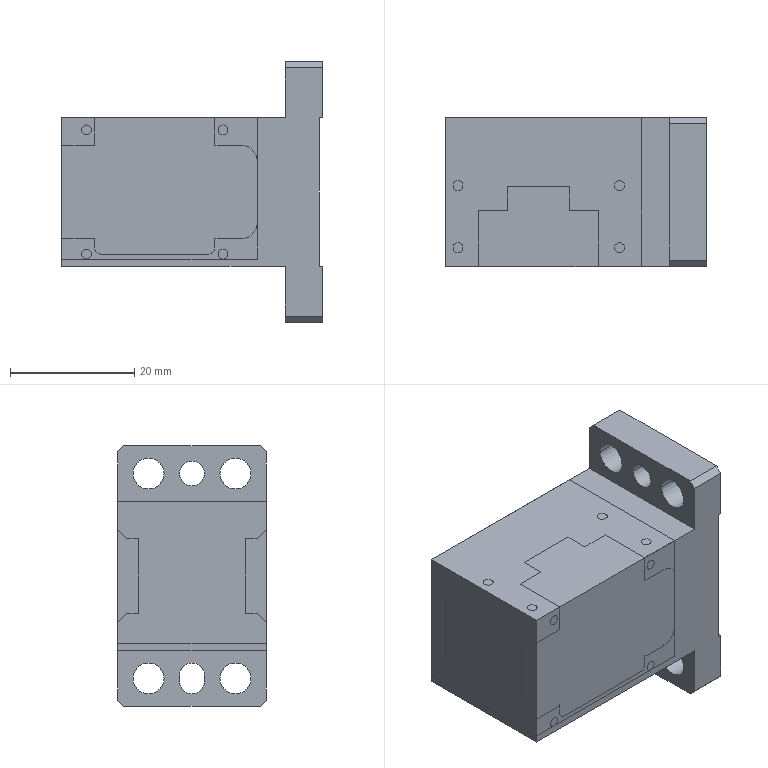NC program | NX | posted with a generic post | part box 42 x 24 x 42 mm
Whole program, first 1893 of 2020 lines:
N10 G17 G21 G94 G90
(DRILLING_COPY_2 , TOOL : ZXZ)
N12 T08 M6
N14 G54
N16 G17 G0 G90 X10. Y-17. B0. C0. S5000 M3
N18 G43 Z30. H8
N20 G94 G81 G98 Z-1.1 F250. R3.
N22 X-10.
N24 Y5.
N26 X10.
N28 G80
N30 G0 X10. Y5. Z30.
N32 M5
(DRILLING_COPY_COPY_1 , TOOL : 1.6ZT)
N34 T16 M6
N36 G54
N38 G17 G0 G90 X10. Y-17. B0. C0. S2000 M3
N40 G43 Z30. H16
N42 G94 G83 G98 Z-5.681 F100. Q2. R3.
N44 X-10.
N46 Y5.
N48 X10.
N50 G80
N52 G0 X10. Y5. Z30.
N54 M5
(FLOOR_WALL_1_COPY_COPY , TOOL : D6)
N56 T06 M6
N58 G54
N60 G17 G0 G90 X1.212 Y-25.5 B0. C0. S4500 M3
N62 G43 Z30. H6
N64 Z1.45
N66 G94 G1 Z-0.05 F1000.
N68 X0.52 Y-24.3
N70 G3 X0. Y-24. R0.6
N72 G1 X-3. F2000.
N74 Y-15.
N76 X3.
N78 Y-24.
N80 X0.
N82 Y-21.
N84 Y-18.
N86 Y-21.
N88 G3 X0.3 Y-21.52 R0.6
N90 G1 Y-25.5
N92 Z1.45
N94 G0 X1.212 Z1.35
N96 G1 Z-0.15 F1000.
N98 X0.52 Y-24.3
N100 G3 X0. Y-24. R0.6
N102 G1 X-3. F2000.
N104 Y-15.
N106 X3.
N108 Y-24.
N110 X0.
N112 Y-21.
N114 Y-18.
N116 Y-21.
N118 G3 X0.3 Y-21.52 R0.6
N120 G1 Y-25.5
N122 Z1.35
N124 G0 X1.212 Z1.25
N126 G1 Z-0.25 F1000.
N128 X0.52 Y-24.3
N130 G3 X0. Y-24. R0.6
N132 G1 X-3. F2000.
N134 Y-15.
N136 X3.
N138 Y-24.
N140 X0.
N142 Y-21.
N144 Y-18.
N146 Y-21.
N148 G3 X0.3 Y-21.52 R0.6
N150 G1 Y-25.5
N152 Z1.25
N154 G0 X1.212 Z1.15
N156 G1 Z-0.35 F1000.
N158 X0.52 Y-24.3
N160 G3 X0. Y-24. R0.6
N162 G1 X-3. F2000.
N164 Y-15.
N166 X3.
N168 Y-24.
N170 X0.
N172 Y-21.
N174 Y-18.
N176 Y-21.
N178 G3 X0.3 Y-21.52 R0.6
N180 G1 Y-25.5
N182 Z1.15
N184 G0 X1.212 Z1.05
N186 G1 Z-0.45 F1000.
N188 X0.52 Y-24.3
N190 G3 X0. Y-24. R0.6
N192 G1 X-3. F2000.
N194 Y-15.
N196 X3.
N198 Y-24.
N200 X0.
N202 Y-21.
N204 Y-18.
N206 Y-21.
N208 G3 X0.3 Y-21.52 R0.6
N210 G1 Y-25.5
N212 Z1.05
N214 G0 X1.212 Z0.95
N216 G1 Z-0.55 F1000.
N218 X0.52 Y-24.3
N220 G3 X0. Y-24. R0.6
N222 G1 X-3. F2000.
N224 Y-15.
N226 X3.
N228 Y-24.
N230 X0.
N232 Y-21.
N234 Y-18.
N236 Y-21.
N238 G3 X0.3 Y-21.52 R0.6
N240 G1 Y-25.5
N242 Z0.95
N244 G0 X1.212 Z0.85
N246 G1 Z-0.65 F1000.
N248 X0.52 Y-24.3
N250 G3 X0. Y-24. R0.6
N252 G1 X-3. F2000.
N254 Y-15.
N256 X3.
N258 Y-24.
N260 X0.
N262 Y-21.
N264 Y-18.
N266 Y-21.
N268 G3 X0.3 Y-21.52 R0.6
N270 G1 Y-25.5
N272 Z0.85
N274 G0 X1.212 Z0.75
N276 G1 Z-0.75 F1000.
N278 X0.52 Y-24.3
N280 G3 X0. Y-24. R0.6
N282 G1 X-3. F2000.
N284 Y-15.
N286 X3.
N288 Y-24.
N290 X0.
N292 Y-21.
N294 Y-18.
N296 Y-21.
N298 G3 X0.3 Y-21.52 R0.6
N300 G1 Y-25.5
N302 Z0.75
N304 G0 X1.212 Z0.65
N306 G1 Z-0.85 F1000.
N308 X0.52 Y-24.3
N310 G3 X0. Y-24. R0.6
N312 G1 X-3. F2000.
N314 Y-15.
N316 X3.
N318 Y-24.
N320 X0.
N322 Y-21.
N324 Y-18.
N326 Y-21.
N328 G3 X0.3 Y-21.52 R0.6
N330 G1 Y-25.5
N332 Z0.65
N334 G0 X1.212 Z0.55
N336 G1 Z-0.95 F1000.
N338 X0.52 Y-24.3
N340 G3 X0. Y-24. R0.6
N342 G1 X-3. F2000.
N344 Y-15.
N346 X3.
N348 Y-24.
N350 X0.
N352 Y-21.
N354 Y-18.
N356 Y-21.
N358 G3 X0.3 Y-21.52 R0.6
N360 G1 Y-25.5
N362 Z0.55
N364 G0 X1.212 Z0.45
N366 G1 Z-1.05 F1000.
N368 X0.52 Y-24.3
N370 G3 X0. Y-24. R0.6
N372 G1 X-3. F2000.
N374 Y-15.
N376 X3.
N378 Y-24.
N380 X0.
N382 Y-21.
N384 Y-18.
N386 Y-21.
N388 G3 X0.3 Y-21.52 R0.6
N390 G1 Y-25.5
N392 Z0.45
N394 G0 X1.212 Z0.35
N396 G1 Z-1.15 F1000.
N398 X0.52 Y-24.3
N400 G3 X0. Y-24. R0.6
N402 G1 X-3. F2000.
N404 Y-15.
N406 X3.
N408 Y-24.
N410 X0.
N412 Y-21.
N414 Y-18.
N416 Y-21.
N418 G3 X0.3 Y-21.52 R0.6
N420 G1 Y-25.5
N422 Z0.35
N424 G0 X1.212 Z0.25
N426 G1 Z-1.25 F1000.
N428 X0.52 Y-24.3
N430 G3 X0. Y-24. R0.6
N432 G1 X-3. F2000.
N434 Y-15.
N436 X3.
N438 Y-24.
N440 X0.
N442 Y-21.
N444 Y-18.
N446 Y-21.
N448 G3 X0.3 Y-21.52 R0.6
N450 G1 Y-25.5
N452 Z0.25
N454 G0 X1.212 Z0.15
N456 G1 Z-1.35 F1000.
N458 X0.52 Y-24.3
N460 G3 X0. Y-24. R0.6
N462 G1 X-3. F2000.
N464 Y-15.
N466 X3.
N468 Y-24.
N470 X0.
N472 Y-21.
N474 Y-18.
N476 Y-21.
N478 G3 X0.3 Y-21.52 R0.6
N480 G1 Y-25.5
N482 Z0.15
N484 G0 X1.212 Z0.05
N486 G1 Z-1.45 F1000.
N488 X0.52 Y-24.3
N490 G3 X0. Y-24. R0.6
N492 G1 X-3. F2000.
N494 Y-15.
N496 X3.
N498 Y-24.
N500 X0.
N502 Y-21.
N504 Y-18.
N506 Y-21.
N508 G3 X0.3 Y-21.52 R0.6
N510 G1 Y-25.5
N512 Z0.05
N514 G0 X1.212 Z-0.05
N516 G1 Z-1.55 F1000.
N518 X0.52 Y-24.3
N520 G3 X0. Y-24. R0.6
N522 G1 X-3. F2000.
N524 Y-15.
N526 X3.
N528 Y-24.
N530 X0.
N532 Y-21.
N534 Y-18.
N536 Y-21.
N538 G3 X0.3 Y-21.52 R0.6
N540 G1 Y-25.5
N542 Z-0.05
N544 G0 X1.212 Z-0.15
N546 G1 Z-1.65 F1000.
N548 X0.52 Y-24.3
N550 G3 X0. Y-24. R0.6
N552 G1 X-3. F2000.
N554 Y-15.
N556 X3.
N558 Y-24.
N560 X0.
N562 Y-21.
N564 Y-18.
N566 Y-21.
N568 G3 X0.3 Y-21.52 R0.6
N570 G1 Y-25.5
N572 Z-0.15
N574 G0 X1.212 Z-0.25
N576 G1 Z-1.75 F1000.
N578 X0.52 Y-24.3
N580 G3 X0. Y-24. R0.6
N582 G1 X-3. F2000.
N584 Y-15.
N586 X3.
N588 Y-24.
N590 X0.
N592 Y-21.
N594 Y-18.
N596 Y-21.
N598 G3 X0.3 Y-21.52 R0.6
N600 G1 Y-25.5
N602 Z-0.25
N604 G0 X1.212 Z-0.35
N606 G1 Z-1.85 F1000.
N608 X0.52 Y-24.3
N610 G3 X0. Y-24. R0.6
N612 G1 X-3. F2000.
N614 Y-15.
N616 X3.
N618 Y-24.
N620 X0.
N622 Y-21.
N624 Y-18.
N626 Y-21.
N628 G3 X0.3 Y-21.52 R0.6
N630 G1 Y-25.5
N632 Z-0.35
N634 G0 X1.212 Z-0.45
N636 G1 Z-1.95 F1000.
N638 X0.52 Y-24.3
N640 G3 X0. Y-24. R0.6
N642 G1 X-3. F2000.
N644 Y-15.
N646 X3.
N648 Y-24.
N650 X0.
N652 Y-21.
N654 Y-18.
N656 Y-21.
N658 G3 X0.3 Y-21.52 R0.6
N660 G1 Y-25.5
N662 Z-0.45
N664 G0 X1.212 Z-0.55
N666 G1 Z-2.05 F1000.
N668 X0.52 Y-24.3
N670 G3 X0. Y-24. R0.6
N672 G1 X-3. F2000.
N674 Y-15.
N676 X3.
N678 Y-24.
N680 X0.
N682 Y-21.
N684 Y-18.
N686 Y-21.
N688 G3 X0.3 Y-21.52 R0.6
N690 G1 Y-25.5
N692 Z-0.55
N694 G0 X1.212 Z-0.65
N696 G1 Z-2.15 F1000.
N698 X0.52 Y-24.3
N700 G3 X0. Y-24. R0.6
N702 G1 X-3. F2000.
N704 Y-15.
N706 X3.
N708 Y-24.
N710 X0.
N712 Y-21.
N714 Y-18.
N716 Y-21.
N718 G3 X0.3 Y-21.52 R0.6
N720 G1 Y-25.5
N722 Z-0.65
N724 G0 X1.212 Z-0.75
N726 G1 Z-2.25 F1000.
N728 X0.52 Y-24.3
N730 G3 X0. Y-24. R0.6
N732 G1 X-3. F2000.
N734 Y-15.
N736 X3.
N738 Y-24.
N740 X0.
N742 Y-21.
N744 Y-18.
N746 Y-21.
N748 G3 X0.3 Y-21.52 R0.6
N750 G1 Y-25.5
N752 Z-0.75
N754 G0 X1.212 Z-0.85
N756 G1 Z-2.35 F1000.
N758 X0.52 Y-24.3
N760 G3 X0. Y-24. R0.6
N762 G1 X-3. F2000.
N764 Y-15.
N766 X3.
N768 Y-24.
N770 X0.
N772 Y-21.
N774 Y-18.
N776 Y-21.
N778 G3 X0.3 Y-21.52 R0.6
N780 G1 Y-25.5
N782 Z-0.85
N784 G0 X1.212 Z-0.95
N786 G1 Z-2.45 F1000.
N788 X0.52 Y-24.3
N790 G3 X0. Y-24. R0.6
N792 G1 X-3. F2000.
N794 Y-15.
N796 X3.
N798 Y-24.
N800 X0.
N802 Y-21.
N804 Y-18.
N806 Y-21.
N808 G3 X0.3 Y-21.52 R0.6
N810 G1 Y-25.5
N812 Z-0.95
N814 G0 X1.212 Z-1.05
N816 G1 Z-2.55 F1000.
N818 X0.52 Y-24.3
N820 G3 X0. Y-24. R0.6
N822 G1 X-3. F2000.
N824 Y-15.
N826 X3.
N828 Y-24.
N830 X0.
N832 Y-21.
N834 Y-18.
N836 Y-21.
N838 G3 X0.3 Y-21.52 R0.6
N840 G1 Y-25.5
N842 Z-1.05
N844 G0 X1.212 Z-1.15
N846 G1 Z-2.65 F1000.
N848 X0.52 Y-24.3
N850 G3 X0. Y-24. R0.6
N852 G1 X-3. F2000.
N854 Y-15.
N856 X3.
N858 Y-24.
N860 X0.
N862 Y-21.
N864 Y-18.
N866 Y-21.
N868 G3 X0.3 Y-21.52 R0.6
N870 G1 Y-25.5
N872 Z-1.15
N874 G0 X1.212 Z-1.25
N876 G1 Z-2.75 F1000.
N878 X0.52 Y-24.3
N880 G3 X0. Y-24. R0.6
N882 G1 X-3. F2000.
N884 Y-15.
N886 X3.
N888 Y-24.
N890 X0.
N892 Y-21.
N894 Y-18.
N896 Y-21.
N898 G3 X0.3 Y-21.52 R0.6
N900 G1 Y-25.5
N902 Z-1.25
N904 G0 X1.212 Z-1.35
N906 G1 Z-2.85 F1000.
N908 X0.52 Y-24.3
N910 G3 X0. Y-24. R0.6
N912 G1 X-3. F2000.
N914 Y-15.
N916 X3.
N918 Y-24.
N920 X0.
N922 Y-21.
N924 Y-18.
N926 Y-21.
N928 G3 X0.3 Y-21.52 R0.6
N930 G1 Y-25.5
N932 Z-1.35
N934 G0 X1.212 Z-1.45
N936 G1 Z-2.95 F1000.
N938 X0.52 Y-24.3
N940 G3 X0. Y-24. R0.6
N942 G1 X-3. F2000.
N944 Y-15.
N946 X3.
N948 Y-24.
N950 X0.
N952 Y-21.
N954 Y-18.
N956 Y-21.
N958 G3 X0.3 Y-21.52 R0.6
N960 G1 Y-25.5
N962 Z-1.45
N964 G0 X1.212 Z-1.55
N966 G1 Z-3.05 F1000.
N968 X0.52 Y-24.3
N970 G3 X0. Y-24. R0.6
N972 G1 X-3. F2000.
N974 Y-15.
N976 X3.
N978 Y-24.
N980 X0.
N982 Y-21.
N984 Y-18.
N986 Y-21.
N988 G3 X0.3 Y-21.52 R0.6
N990 G1 Y-25.5
N992 Z-1.55
N994 G0 X1.212 Z-1.65
N996 G1 Z-3.15 F1000.
N998 X0.52 Y-24.3
N1000 G3 X0. Y-24. R0.6
N1002 G1 X-3. F2000.
N1004 Y-15.
N1006 X3.
N1008 Y-24.
N1010 X0.
N1012 Y-21.
N1014 Y-18.
N1016 Y-21.
N1018 G3 X0.3 Y-21.52 R0.6
N1020 G1 Y-25.5
N1022 Z-1.65
N1024 G0 X1.212 Z-1.75
N1026 G1 Z-3.25 F1000.
N1028 X0.52 Y-24.3
N1030 G3 X0. Y-24. R0.6
N1032 G1 X-3. F2000.
N1034 Y-15.
N1036 X3.
N1038 Y-24.
N1040 X0.
N1042 Y-21.
N1044 Y-18.
N1046 Y-21.
N1048 G3 X0.3 Y-21.52 R0.6
N1050 G1 Y-25.5
N1052 Z-1.75
N1054 G0 X1.212 Z-1.85
N1056 G1 Z-3.35 F1000.
N1058 X0.52 Y-24.3
N1060 G3 X0. Y-24. R0.6
N1062 G1 X-3. F2000.
N1064 Y-15.
N1066 X3.
N1068 Y-24.
N1070 X0.
N1072 Y-21.
N1074 Y-18.
N1076 Y-21.
N1078 G3 X0.3 Y-21.52 R0.6
N1080 G1 Y-25.5
N1082 Z-1.85
N1084 G0 Z30.
N1086 X2.7 Y2.48
N1088 Z1.45
N1090 G1 Z-0.05 F1000.
N1092 G3 X3. Y3. R0.6
N1094 G1 Y6. F2000.
N1096 X-3.
N1098 Y3.
N1100 G3 X-2.7 Y2.48 R0.6
N1102 G1 Z1.45
N1104 G0 X2.7 Z1.35
N1106 G1 Z-0.15 F1000.
N1108 G3 X3. Y3. R0.6
N1110 G1 Y6. F2000.
N1112 X-3.
N1114 Y3.
N1116 G3 X-2.7 Y2.48 R0.6
N1118 G1 Z1.35
N1120 G0 X2.7 Z1.25
N1122 G1 Z-0.25 F1000.
N1124 G3 X3. Y3. R0.6
N1126 G1 Y6. F2000.
N1128 X-3.
N1130 Y3.
N1132 G3 X-2.7 Y2.48 R0.6
N1134 G1 Z1.25
N1136 G0 X2.65 Y2.452 Z1.15
N1138 G1 Z-0.35 F1000.
N1140 X2.7 Y2.48
N1142 G3 X3. Y3. R0.6
N1144 G1 Y6. F2000.
N1146 X-3.
N1148 Y3.
N1150 G3 X-2.65 Y2.452 R0.603
N1152 G1 Z1.15
N1154 G0 X2.55 Y2.394 Z1.05
N1156 G1 Z-0.45 F1000.
N1158 X2.7 Y2.48
N1160 G3 X3. Y3. R0.6
N1162 G1 Y6. F2000.
N1164 X-3.
N1166 Y3.
N1168 G3 X-2.7 Y2.48 R0.6
N1170 G1 X-2.55 Y2.394
N1172 Z1.05
N1174 G0 X2.45 Y2.336 Z0.95
N1176 G1 Z-0.55 F1000.
N1178 X2.7 Y2.48
N1180 G3 X3. Y3. R0.6
N1182 G1 Y6. F2000.
N1184 X-3.
N1186 Y3.
N1188 G3 X-2.7 Y2.48 R0.6
N1190 G1 X-2.45 Y2.336
N1192 Z0.95
N1194 G0 X2.35 Y2.278 Z0.85
N1196 G1 Z-0.65 F1000.
N1198 X2.7 Y2.48
N1200 G3 X3. Y3. R0.6
N1202 G1 Y6. F2000.
N1204 X-3.
N1206 Y3.
N1208 G3 X-2.7 Y2.48 R0.6
N1210 G1 X-2.35 Y2.278
N1212 Z0.85
N1214 G0 X2.25 Y2.221 Z0.75
N1216 G1 Z-0.75 F1000.
N1218 X2.7 Y2.48
N1220 G3 X3. Y3. R0.6
N1222 G1 Y6. F2000.
N1224 X-3.
N1226 Y3.
N1228 G3 X-2.7 Y2.48 R0.6
N1230 G1 X-2.25 Y2.221
N1232 Z0.75
N1234 G0 X2.15 Y2.163 Z0.65
N1236 G1 Z-0.85 F1000.
N1238 X2.7 Y2.48
N1240 G3 X3. Y3. R0.6
N1242 G1 Y6. F2000.
N1244 X-3.
N1246 Y3.
N1248 G3 X-2.7 Y2.48 R0.6
N1250 G1 X-2.15 Y2.163
N1252 Z0.65
N1254 G0 X2.05 Y2.105 Z0.55
N1256 G1 Z-0.95 F1000.
N1258 X2.7 Y2.48
N1260 G3 X3. Y3. R0.6
N1262 G1 Y6. F2000.
N1264 X-3.
N1266 Y3.
N1268 G3 X-2.7 Y2.48 R0.6
N1270 G1 X-2.05 Y2.105
N1272 Z0.55
N1274 G0 X1.95 Y2.047 Z0.45
N1276 G1 Z-1.05 F1000.
N1278 X2.7 Y2.48
N1280 G3 X3. Y3. R0.6
N1282 G1 Y6. F2000.
N1284 X-3.
N1286 Y3.
N1288 G3 X-2.7 Y2.48 R0.6
N1290 G1 X-1.95 Y2.047
N1292 Z0.45
N1294 G0 X1.85 Y1.99 Z0.35
N1296 G1 Z-1.15 F1000.
N1298 X2.7 Y2.48
N1300 G3 X3. Y3. R0.6
N1302 G1 Y6. F2000.
N1304 X-3.
N1306 Y3.
N1308 G3 X-2.7 Y2.48 R0.6
N1310 G1 X-1.85 Y1.99
N1312 Z0.35
N1314 G0 X1.75 Y1.932 Z0.25
N1316 G1 Z-1.25 F1000.
N1318 X2.7 Y2.48
N1320 G3 X3. Y3. R0.6
N1322 G1 Y6. F2000.
N1324 X-3.
N1326 Y3.
N1328 G3 X-2.7 Y2.48 R0.6
N1330 G1 X-1.75 Y1.932
N1332 Z0.25
N1334 G0 X1.65 Y1.874 Z0.15
N1336 G1 Z-1.35 F1000.
N1338 X2.7 Y2.48
N1340 G3 X3. Y3. R0.6
N1342 G1 Y6. F2000.
N1344 X-3.
N1346 Y3.
N1348 G3 X-2.7 Y2.48 R0.6
N1350 G1 X-1.65 Y1.874
N1352 Z0.15
N1354 G0 X1.55 Y1.816 Z0.05
N1356 G1 Z-1.45 F1000.
N1358 X2.7 Y2.48
N1360 G3 X3. Y3. R0.6
N1362 G1 Y6. F2000.
N1364 X-3.
N1366 Y3.
N1368 G3 X-2.7 Y2.48 R0.6
N1370 G1 X-1.55 Y1.816
N1372 Z0.05
N1374 G0 X1.5 Y1.788 Z-0.05
N1376 G1 Z-1.55 F1000.
N1378 X2.7 Y2.48
N1380 G3 X3. Y3. R0.6
N1382 G1 Y6. F2000.
N1384 X-3.
N1386 Y3.
N1388 G3 X-2.7 Y2.48 R0.6
N1390 G1 X-1.5 Y1.788
N1392 Z-0.05
N1394 G0 X1.5 Z-0.15
N1396 G1 Z-1.65 F1000.
N1398 X2.7 Y2.48
N1400 G3 X3. Y3. R0.6
N1402 G1 Y6. F2000.
N1404 X-3.
N1406 Y3.
N1408 G3 X-2.7 Y2.48 R0.6
N1410 G1 X-1.5 Y1.788
N1412 Z-0.15
N1414 G0 X1.5 Z-0.25
N1416 G1 Z-1.75 F1000.
N1418 X2.7 Y2.48
N1420 G3 X3. Y3. R0.6
N1422 G1 Y6. F2000.
N1424 X-3.
N1426 Y3.
N1428 G3 X-2.7 Y2.48 R0.6
N1430 G1 X-1.5 Y1.788
N1432 Z-0.25
N1434 G0 X1.5 Z-0.35
N1436 G1 Z-1.85 F1000.
N1438 X2.7 Y2.48
N1440 G3 X3. Y3. R0.6
N1442 G1 Y6. F2000.
N1444 X-3.
N1446 Y3.
N1448 G3 X-2.7 Y2.48 R0.6
N1450 G1 X-1.5 Y1.788
N1452 Z-0.35
N1454 G0 X1.5 Z-0.45
N1456 G1 Z-1.95 F1000.
N1458 X2.7 Y2.48
N1460 G3 X3. Y3. R0.6
N1462 G1 Y6. F2000.
N1464 X-3.
N1466 Y3.
N1468 G3 X-2.7 Y2.48 R0.6
N1470 G1 X-1.5 Y1.788
N1472 Z-0.45
N1474 G0 X1.5 Z-0.55
N1476 G1 Z-2.05 F1000.
N1478 X2.7 Y2.48
N1480 G3 X3. Y3. R0.6
N1482 G1 Y6. F2000.
N1484 X-3.
N1486 Y3.
N1488 G3 X-2.7 Y2.48 R0.6
N1490 G1 X-1.5 Y1.788
N1492 Z-0.55
N1494 G0 X1.5 Z-0.65
N1496 G1 Z-2.15 F1000.
N1498 X2.7 Y2.48
N1500 G3 X3. Y3. R0.6
N1502 G1 Y6. F2000.
N1504 X-3.
N1506 Y3.
N1508 G3 X-2.7 Y2.48 R0.6
N1510 G1 X-1.5 Y1.788
N1512 Z-0.65
N1514 G0 X1.5 Z-0.75
N1516 G1 Z-2.25 F1000.
N1518 X2.7 Y2.48
N1520 G3 X3. Y3. R0.6
N1522 G1 Y6. F2000.
N1524 X-3.
N1526 Y3.
N1528 G3 X-2.7 Y2.48 R0.6
N1530 G1 X-1.5 Y1.788
N1532 Z-0.75
N1534 G0 X1.5 Z-0.85
N1536 G1 Z-2.35 F1000.
N1538 X2.7 Y2.48
N1540 G3 X3. Y3. R0.6
N1542 G1 Y6. F2000.
N1544 X-3.
N1546 Y3.
N1548 G3 X-2.7 Y2.48 R0.6
N1550 G1 X-1.5 Y1.788
N1552 Z-0.85
N1554 G0 X1.5 Z-0.95
N1556 G1 Z-2.45 F1000.
N1558 X2.7 Y2.48
N1560 G3 X3. Y3. R0.6
N1562 G1 Y6. F2000.
N1564 X-3.
N1566 Y3.
N1568 G3 X-2.7 Y2.48 R0.6
N1570 G1 X-1.5 Y1.788
N1572 Z-0.95
N1574 G0 X1.5 Z-1.05
N1576 G1 Z-2.55 F1000.
N1578 X2.7 Y2.48
N1580 G3 X3. Y3. R0.6
N1582 G1 Y6. F2000.
N1584 X-3.
N1586 Y3.
N1588 G3 X-2.7 Y2.48 R0.6
N1590 G1 X-1.5 Y1.788
N1592 Z-1.05
N1594 G0 X1.5 Z-1.15
N1596 G1 Z-2.65 F1000.
N1598 X2.7 Y2.48
N1600 G3 X3. Y3. R0.6
N1602 G1 Y6. F2000.
N1604 X-3.
N1606 Y3.
N1608 G3 X-2.7 Y2.48 R0.6
N1610 G1 X-1.5 Y1.788
N1612 Z-1.15
N1614 G0 X1.5 Z-1.25
N1616 G1 Z-2.75 F1000.
N1618 X2.7 Y2.48
N1620 G3 X3. Y3. R0.6
N1622 G1 Y6. F2000.
N1624 X-3.
N1626 Y3.
N1628 G3 X-2.7 Y2.48 R0.6
N1630 G1 X-1.5 Y1.788
N1632 Z-1.25
N1634 G0 X1.5 Z-1.35
N1636 G1 Z-2.85 F1000.
N1638 X2.7 Y2.48
N1640 G3 X3. Y3. R0.6
N1642 G1 Y6. F2000.
N1644 X-3.
N1646 Y3.
N1648 G3 X-2.7 Y2.48 R0.6
N1650 G1 X-1.5 Y1.788
N1652 Z-1.35
N1654 G0 X1.5 Z-1.45
N1656 G1 Z-2.95 F1000.
N1658 X2.7 Y2.48
N1660 G3 X3. Y3. R0.6
N1662 G1 Y6. F2000.
N1664 X-3.
N1666 Y3.
N1668 G3 X-2.7 Y2.48 R0.6
N1670 G1 X-1.5 Y1.788
N1672 Z-1.45
N1674 G0 X1.5 Z-1.55
N1676 G1 Z-3.05 F1000.
N1678 X2.7 Y2.48
N1680 G3 X3. Y3. R0.6
N1682 G1 Y6. F2000.
N1684 X-3.
N1686 Y3.
N1688 G3 X-2.7 Y2.48 R0.6
N1690 G1 X-1.5 Y1.788
N1692 Z-1.55
N1694 G0 X1.5 Z-1.65
N1696 G1 Z-3.15 F1000.
N1698 X2.7 Y2.48
N1700 G3 X3. Y3. R0.6
N1702 G1 Y6. F2000.
N1704 X-3.
N1706 Y3.
N1708 G3 X-2.7 Y2.48 R0.6
N1710 G1 X-1.5 Y1.788
N1712 Z-1.65
N1714 G0 X1.5 Z-1.75
N1716 G1 Z-3.25 F1000.
N1718 X2.7 Y2.48
N1720 G3 X3. Y3. R0.6
N1722 G1 Y6. F2000.
N1724 X-3.
N1726 Y3.
N1728 G3 X-2.7 Y2.48 R0.6
N1730 G1 X-1.5 Y1.788
N1732 Z-1.75
N1734 G0 X1.5 Z-1.85
N1736 G1 Z-3.35 F1000.
N1738 X2.7 Y2.48
N1740 G3 X3. Y3. R0.6
N1742 G1 Y6. F2000.
N1744 X-3.
N1746 Y3.
N1748 G3 X-2.7 Y2.48 R0.6
N1750 G1 X-1.5 Y1.788
N1752 Z-1.85
N1754 G0 Z30.
N1756 M5
(ZLEVEL_PROFILE_2_COPY , TOOL : D4R0.5)
N1758 T05 M6
N1760 G54
N1762 G17 G0 G90 X5.003 Y-22.118 B0. C0. S6500 M3
N1764 G43 Z30. H5
N1766 Z0.929
N1768 G94 G1 Z-0.071 F3000.
N1770 X5.523 Y-21.818
N1772 G3 X5.723 Y-21.472 R0.4
N1774 G1 X5.722 Y6.467
N1776 X5.712 Y7.877
N1778 G3 X5.664 Y8.201 R1.173
N1780 X5.069 Y8.694 R0.694
N1782 G1 X4.911 Y8.71
N1784 X3.508 Y8.719
N1786 X-4.069 Y8.722
N1788 X-4.911 Y8.712
N1790 X-5.051 Y8.698
N1792 G3 X-5.699 Y8.018 R0.716
N1794 G1 X-5.71 Y7.877
N1796 X-5.721 Y5.902
N1798 X-5.723 Y-21.472
N1800 X-5.687 Z-0.106
N1802 X-5.652 Z-0.141
N1804 X-5.649 Y7.877
N1806 G2 X-5.61 Y8.174 R0.981
N1808 X-4.976 Y8.65 R0.661
N1810 G1 X3.227 Y8.651
N1812 X4.982 Y8.648
N1814 G2 X5.608 Y8.184 R0.655
N1816 X5.651 Y7.877 R0.993
N1818 G1 X5.652 Y-21.472
N1820 X5.616 Z-0.177
N1822 X5.582 Z-0.212
N1824 X5.581 Y-21.
N1826 Y8.
N1828 G3 X5. Y8.581 R0.581
N1830 G1 X-5.
N1832 G3 X-5.581 Y8. R0.581
N1834 G1 Y-21.
N1836 Y-21.472
N1838 X-5.545 Z-0.247
N1840 X-5.511 Z-0.283
N1842 X-5.51 Y-21.
N1844 Y8.
N1846 G2 X-5. Y8.51 R0.51
N1848 G1 X5.
N1850 G2 X5.51 Y8. R0.51
N1852 G1 Y-21.
N1854 X5.511 Y-21.472
N1856 X5.475 Z-0.318
N1858 X5.44 Z-0.354
N1860 X5.439 Y-21.
N1862 Y8.
N1864 G3 X5. Y8.439 R0.439
N1866 G1 X-5.
N1868 G3 X-5.439 Y8. R0.439
N1870 G1 Y-21.
N1872 X-5.44 Y-21.472
N1874 X-5.404 Z-0.389
N1876 X-5.369 Z-0.424
N1878 Y-21.
N1880 Y8.
N1882 G2 X-5. Y8.369 R0.369
N1884 G1 X5.
N1886 G2 X5.369 Y8. R0.369
N1888 G1 Y-21.
N1890 Y-21.472
N1892 X5.333 Z-0.46
N1894 X5.299 Z-0.495
N1896 X5.298 Y-21.
N1898 Y8.
N1900 G3 X5. Y8.298 R0.298
N1902 G1 X-5.
N1904 G3 X-5.298 Y8. R0.298
N1906 G1 Y-21.
N1908 X-5.299 Y-21.472
N1910 X-5.263 Z-0.53
N1912 X-5.228 Z-0.566
N1914 X-5.227 Y-21.
N1916 Y8.
N1918 G2 X-5. Y8.227 R0.227
N1920 G1 X5.
N1922 G2 X5.227 Y8. R0.227
N1924 G1 Y-21.
N1926 X5.228 Y-21.472
N1928 X5.192 Z-0.601
N1930 X5.157 Z-0.636
N1932 X5.156 Y-21.
N1934 Y8.
N1936 G3 X5. Y8.156 R0.156
N1938 G1 X-5.
N1940 G3 X-5.156 Y8. R0.156
N1942 G1 Y-21.
N1944 X-5.157 Y-21.472
N1946 X-5.121 Z-0.672
N1948 X-5.087 Z-0.707
N1950 X-5.086 Y-21.
N1952 Y8.
N1954 X-5.083 Y8.048
N1956 X-5.048 Y8.083
N1958 X-5. Y8.086
N1960 X5.
N1962 X5.048 Y8.083
N1964 X5.083 Y8.048
N1966 X5.086 Y8.
N1968 Y-21.
N1970 X5.087 Y-21.472
N1972 X5.05 Z-0.742
N1974 X5.016 Z-0.778
N1976 X5.015 Y-21.
N1978 Y8.
N1980 X5.016 Y8.016
N1982 X5. Y8.015
N1984 X-5.
N1986 X-5.016 Y8.016
N1988 X-5.015 Y8.
N1990 Y-21.
N1992 X-5.016 Y-21.472
N1994 X-4.98 Z-0.813
N1996 X-4.945 Z-0.849
N1998 X-4.944 Y-21.
N2000 Y7.944
N2002 X4.944
N2004 Y-21.
N2006 X4.945 Y-21.472
N2008 X4.909 Z-0.884
N2010 X4.874 Z-0.919
N2012 Y-21.
N2014 Y7.874
N2016 X-4.874
N2018 Y-21.
N2020 Y-21.472
N2022 X-4.838 Z-0.955
N2024 X-4.804 Z-0.99
N2026 X-4.803 Y-21.
N2028 Y7.803
N2030 X4.803
N2032 Y-21.
N2034 X4.804 Y-21.472
N2036 X4.768 Z-1.025
N2038 X4.733 Z-1.061
N2040 X4.732 Y-21.
N2042 Y7.732
N2044 X-4.732
N2046 Y-21.
N2048 X-4.733 Y-21.472
N2050 X-4.697 Z-1.096
N2052 X-4.662 Z-1.131
N2054 Y-21.
N2056 Y7.662
N2058 X4.662
N2060 Y-21.
N2062 Y-21.472
N2064 X4.626 Z-1.167
N2066 X4.592 Z-1.202
N2068 X4.591 Y-21.
N2070 Y7.591
N2072 X-4.591
N2074 Y-21.
N2076 Y-21.472
N2078 X-4.555 Z-1.237
N2080 X-4.521 Z-1.273
N2082 X-4.52 Y-21.
N2084 Y7.52
N2086 X4.52
N2088 Y-21.
N2090 X4.521 Y-21.472
N2092 X4.485 Z-1.308
N2094 X4.45 Z-1.344
N2096 X4.449 Y-21.
N2098 Y7.449
N2100 X-4.449
N2102 Y-21.
N2104 X-4.45 Y-21.472
N2106 X-4.414 Z-1.379
N2108 X-4.379 Z-1.414
N2110 Y-21.
N2112 Y7.379
N2114 X4.379
N2116 Y-21.
N2118 Y-21.472
N2120 X4.343 Z-1.45
N2122 X4.309 Z-1.485
N2124 X4.308 Y-21.
N2126 Y7.308
N2128 X-4.308
N2130 Y-21.
N2132 X-4.309 Y-21.472
N2134 X-4.273 Z-1.52
N2136 X-4.238 Z-1.556
N2138 X-4.237 Y-21.
N2140 Y7.237
N2142 X4.237
N2144 Y-21.
N2146 X4.238 Y-21.472
N2148 X4.202 Z-1.591
N2150 X4.167 Z-1.626
N2152 Y-21.
N2154 Y7.167
N2156 X-4.167
N2158 Y-21.
N2160 Y-21.472
N2162 X-4.131 Z-1.661
N2164 X-4.097 Z-1.696
N2166 X-4.093 Y7.093
N2168 X-3.508 Y7.095
N2170 X4.069 Y7.096
N2172 X4.093 Y7.093
N2174 X4.097 Y-21.472
N2176 X4.061 Y-21.471 Z-1.732
N2178 X4.026 Y-21.47 Z-1.767
N2180 X4.025 Y6.184
N2182 X4.02 Y7.021
N2184 X3.789 Y7.025
N2186 X-3.227
N2188 X-4.021 Y7.02
N2190 X-4.026 Y-21.47
N2192 X-3.997 Y-21.469 Z-1.796
N2194 X-3.968 Y-21.468 Z-1.825
N2196 X-3.965 Y6.749
N2198 X-3.961 Y6.962
N2200 X-3.508 Y6.965
N2202 X3.789 Y6.966
N2204 X3.962 Y6.962
N2206 X3.966 Y6.184
N2208 X3.968 Y-21.468
N2210 X3.938 Y-21.467 Z-1.854
N2212 X3.91 Y-21.466 Z-1.884
N2214 X3.908 Y6.184
N2216 X3.904 Y6.903
N2218 X3.789 Y6.906
N2220 X-3.227 Y6.908
N2222 X-3.902 Y6.905
N2224 X-3.91 Y-21.466
N2226 X-3.88 Y-21.465 Z-1.913
N2228 X-3.851 Y-21.464 Z-1.942
N2230 X-3.849 Y6.184
N2232 X-3.843 Y6.847
N2234 X-3.508 Y6.849
N2236 X3.227
N2238 X3.846 Y6.844
N2240 X3.85 Y5.902
N2242 X3.851 Y-21.464
N2244 G2 X3.651 Y-21.81 R0.4
N2246 G1 X3.132 Y-22.11
N2248 Z-0.942
N2250 G0 Z30.
N2252 X2.993 Y-8.896
N2254 Z-1.
N2256 G1 Z-2.
N2258 X3.593 Y-8.55
N2260 G3 X3.793 Y-8.203 R0.4
N2262 G1 X3.792 Y5.902
N2264 X3.788 Y6.784
N2266 X3.227 Y6.791
N2268 X-3.508
N2270 X-3.783 Y6.789
N2272 X-3.79 Y6.184
N2274 X-3.793 Y-8.485
N2276 G3 X-3.593 Y-8.832 R0.4
N2278 G1 X-2.993 Y-9.178
N2280 Z-1.
N2282 G0 Z30.
N2284 M5
(CAVITY_MILL_COPY_COPY , TOOL : D2)
N2286 T02 M6
N2288 G54
N2290 G17 G0 G90 X4.521 Y6.568 B0. C0. S5500 M3
N2292 G43 Z30. H2
N2294 Z-0.45
N2296 G94 G1 Z-0.95 F1000.
N2298 G3 X5.021 Y7.434 R1.
N2300 G1 Y8.001 F800.
N2302 X5.023 Y8.022
N2304 X5.002 Y8.021
N2306 X4.941
N2308 X4.434
N2310 G3 X4.591 Y7.657 R0.5
N2312 X5.15 Y7.394 R1.
N2314 G1 Z-0.45
N2316 G0 X4.521 Y6.463 Z-0.5
N2318 G1 Z-1. F1000.
N2320 G3 X5.021 Y7.329 R1.
N2322 G1 Y8.001 F800.
N2324 X5.023 Y8.022
N2326 X5.002 Y8.021
N2328 X4.941
N2330 X4.329
N2332 G3 X4.5 Y7.645 R0.5
N2334 X5.1 Y7.4 R1.
N2336 G1 Z-0.5
N2338 G0 X4.521 Y6.353 Z-0.55
N2340 G1 Z-1.05 F1000.
N2342 G3 X5.021 Y7.219 R1.
N2344 G1 Y8.001 F800.
N2346 X5.023 Y8.022
N2348 X5.002 Y8.021
N2350 X4.941
N2352 X4.219
N2354 G3 X4.405 Y7.632 R0.5
N2356 X5.05 Y7.411 R1.
N2358 G1 Z-0.55
N2360 G0 X5. Y6.899 Z-0.6
N2362 G1 Z-1.1 F1000.
N2364 G3 X5.021 Y7.105 R1.
N2366 G1 Y8.001 F800.
N2368 X5.023 Y8.022
N2370 X5.002 Y8.021
N2372 X4.941
N2374 X4.105
N2376 G3 X4.306 Y7.62 R0.5
N2378 X5. Y7.428 R1.
N2380 G1 Z-0.6
N2382 G0 X4.95 Y6.615 Z-0.65
N2384 G1 Z-1.15 F1000.
N2386 G3 X5.021 Y6.984 R1.
N2388 G1 Y7.026 F800.
N2390 Y8.001
N2392 X5.023 Y8.022
N2394 X5.002 Y8.021
N2396 X4.941
N2398 X3.984
N2400 G3 X4.204 Y7.608 R0.5
N2402 X4.95 Y7.452 R1.
N2404 G1 Z-0.65
N2406 G0 X4.9 Y6.381 Z-0.7
N2408 G1 Z-1.2 F1000.
N2410 G3 X5.021 Y6.857 R1.
N2412 G1 Y7.026 F800.
N2414 Y8.001
N2416 X5.023 Y8.022
N2418 X5.002 Y8.021
N2420 X4.941
N2422 X3.857
N2424 G3 X4.095 Y7.595 R0.5
N2426 X4.9 Y7.488 R1.
N2428 G1 Z-0.7
N2430 G0 X4.85 Y6.163 Z-0.75
N2432 G1 Z-1.25 F1000.
N2434 G3 X5.021 Y6.721 R1.
N2436 G1 Y7.026 F800.
N2438 Y8.001
N2440 X5.023 Y8.022
N2442 X5.002 Y8.021
N2444 X4.941
N2446 X3.721
N2448 G3 X3.98 Y7.583 R0.5
N2450 X4.85 Y7.539 R1.
N2452 G1 Z-0.75
N2454 G0 X4.8 Y5.948 Z-0.8
N2456 G1 Z-1.3 F1000.
N2458 G3 X5.021 Y6.573 R1.
N2460 G1 Y7.026 F800.
N2462 Y8.001
N2464 X5.023 Y8.022
N2466 X5.002 Y8.021
N2468 X4.941
N2470 X3.573
N2472 G3 X3.857 Y7.571 R0.5
N2474 X4.8 Y7.613 R1.
N2476 G1 Z-0.8
N2478 G0 X4.75 Y5.727 Z-0.85
N2480 G1 Z-1.35 F1000.
N2482 G3 X5.02 Y6.411 R1.
N2484 G1 X5.021 Y7.026 F800.
N2486 Y8.001
N2488 X5.023 Y8.022
N2490 X5.002 Y8.021
N2492 X4.941
N2494 X3.41
N2496 G3 X3.722 Y7.558 R0.5
N2498 X4.713 Y7.696 R1.
N2500 G1 Z-0.85
N2502 G0 X4.7 Y5.491 Z-0.9
N2504 G1 Z-1.4 F1000.
N2506 G3 X5.02 Y6.225 R1.
N2508 G1 Y6.429 F800.
N2510 X5.021 Y7.026
N2512 Y8.001
N2514 X5.023 Y8.022
N2516 X5.002 Y8.021
N2518 X4.941
N2520 X3.223
N2522 G3 X3.569 Y7.546 R0.5
N2524 X4.481 Y7.7 R1.
N2526 G1 Z-0.9
N2528 G0 X4.65 Y5.124 Z-0.95
N2530 G1 Z-1.45 F1000.
N2532 G3 X5.021 Y5.994 R1.
N2534 G1 X5.02 Y6.429 F800.
N2536 X5.021 Y7.026
N2538 Y8.001
N2540 X5.023 Y8.022
N2542 X5.002 Y8.021
N2544 X4.941
N2546 X2.99
N2548 G3 X3.381 Y7.533 R0.5
N2550 X4.11 Y7.65 R1.
N2552 G1 Z-0.95
N2554 G0 X4.6 Y4.984 Z-1.
N2556 G1 Z-1.5 F1000.
N2558 G3 X5. Y5.784 R1.
N2560 G1 Y7.921 F800.
N2562 X5.001 Y8.001
N2564 X4.941 Y8.
N2566 X2.784
N2568 G3 X1.984 Y7.6 R1.
N2570 G1 Z-1.
N2572 G0 X4.6 Y4.984 Z-1.05
N2574 G1 Z-1.55 F1000.
N2576 G3 X5. Y5.784 R1.
N2578 G1 Y7.921 F800.
N2580 X5.001 Y8.001
N2582 X4.941 Y8.
N2584 X2.784
N2586 G3 X1.984 Y7.6 R1.
N2588 G1 Z-1.05
N2590 G0 X4.6 Y4.984 Z-1.1
N2592 G1 Z-1.6 F1000.
N2594 G3 X5. Y5.784 R1.
N2596 G1 Y7.921 F800.
N2598 X5.001 Y8.001
N2600 X4.941 Y8.
N2602 X2.784
N2604 G3 X1.984 Y7.6 R1.
N2606 G1 Z-1.1
N2608 G0 X4.6 Y4.984 Z-1.15
N2610 G1 Z-1.65 F1000.
N2612 G3 X5. Y5.784 R1.
N2614 G1 Y7.921 F800.
N2616 X5.001 Y8.001
N2618 X4.941 Y8.
N2620 X2.784
N2622 G3 X1.984 Y7.6 R1.
N2624 G1 Z-1.15
N2626 G0 X4.6 Y4.984 Z-1.2
N2628 G1 Z-1.7 F1000.
N2630 G3 X5. Y5.784 R1.
N2632 G1 Y7.921 F800.
N2634 X5.001 Y8.001
N2636 X4.941 Y8.
N2638 X2.784
N2640 G3 X1.984 Y7.6 R1.
N2642 G1 Z-1.2
N2644 G0 X4.6 Y4.984 Z-1.25
N2646 G1 Z-1.75 F1000.
N2648 G3 X5. Y5.784 R1.
N2650 G1 Y7.921 F800.
N2652 X5.001 Y8.001
N2654 X4.941 Y8.
N2656 X2.784
N2658 G3 X1.984 Y7.6 R1.
N2660 G1 Z-1.25
N2662 G0 X4.6 Y4.984 Z-1.3
N2664 G1 Z-1.8 F1000.
N2666 G3 X5. Y5.784 R1.
N2668 G1 Y7.921 F800.
N2670 X5.001 Y8.001
N2672 X4.941 Y8.
N2674 X2.784
N2676 G3 X1.984 Y7.6 R1.
N2678 G1 Z-1.3
N2680 G0 X4.6 Y4.984 Z-1.35
N2682 G1 Z-1.85 F1000.
N2684 G3 X5. Y5.784 R1.
N2686 G1 Y7.921 F800.
N2688 X5.001 Y8.001
N2690 X4.941 Y8.
N2692 X2.784
N2694 G3 X1.984 Y7.6 R1.
N2696 G1 Z-1.35
N2698 G0 X4.6 Y4.984 Z-1.4
N2700 G1 Z-1.9 F1000.
N2702 G3 X5. Y5.784 R1.
N2704 G1 Y7.921 F800.
N2706 X5.001 Y8.001
N2708 X4.941 Y8.
N2710 X2.784
N2712 G3 X1.984 Y7.6 R1.
N2714 G1 Z-1.4
N2716 G0 X4.6 Y4.984 Z-1.45
N2718 G1 Z-1.95 F1000.
N2720 G3 X5. Y5.784 R1.
N2722 G1 Y7.921 F800.
N2724 X5.001 Y8.001
N2726 X4.941 Y8.
N2728 X2.784
N2730 G3 X1.984 Y7.6 R1.
N2732 G1 Z-1.45
N2734 G0 X4.6 Y4.984 Z-1.5
N2736 G1 Z-2. F1000.
N2738 G3 X5. Y5.784 R1.
N2740 G1 Y7.921 F800.
N2742 X5.001 Y8.001
N2744 X4.941 Y8.
N2746 X2.784
N2748 G3 X1.984 Y7.6 R1.
N2750 G1 Z-1.5
N2752 G0 X4.6 Y4.984 Z-1.55
N2754 G1 Z-2.05 F1000.
N2756 G3 X5. Y5.784 R1.
N2758 G1 Y7.921 F800.
N2760 X5.001 Y8.001
N2762 X4.941 Y8.
N2764 X2.784
N2766 G3 X1.984 Y7.6 R1.
N2768 G1 Z-1.55
N2770 G0 X4.6 Y4.984 Z-1.6
N2772 G1 Z-2.1 F1000.
N2774 G3 X5. Y5.784 R1.
N2776 G1 Y7.921 F800.
N2778 X5.001 Y8.001
N2780 X4.941 Y8.
N2782 X2.784
N2784 G3 X1.984 Y7.6 R1.
N2786 G1 Z-1.6
N2788 G0 X4.6 Y4.984 Z-1.65
N2790 G1 Z-2.15 F1000.
N2792 G3 X5. Y5.784 R1.
N2794 G1 Y7.921 F800.
N2796 X5.001 Y8.001
N2798 X4.941 Y8.
N2800 X2.784
N2802 G3 X1.984 Y7.6 R1.
N2804 G1 Z-1.65
N2806 G0 X4.6 Y4.984 Z-1.7
N2808 G1 Z-2.2 F1000.
N2810 G3 X5. Y5.784 R1.
N2812 G1 Y7.921 F800.
N2814 X5.001 Y8.001
N2816 X4.941 Y8.
N2818 X2.784
N2820 G3 X1.984 Y7.6 R1.
N2822 G1 Z-1.7
N2824 G0 X4.6 Y4.984 Z-1.75
N2826 G1 Z-2.25 F1000.
N2828 G3 X5. Y5.784 R1.
N2830 G1 Y7.921 F800.
N2832 Y8.
N2834 X4.941
N2836 X2.784
N2838 G3 X1.984 Y7.6 R1.
N2840 G1 Z-1.75
N2842 G0 X4.6 Y4.984 Z-1.8
N2844 G1 Z-2.3 F1000.
N2846 G3 X5. Y5.784 R1.
N2848 G1 Y7.921 F800.
N2850 Y8.
N2852 X4.941
N2854 X2.784
N2856 G3 X1.984 Y7.6 R1.
N2858 G1 Z-1.8
N2860 G0 X4.6 Y4.984 Z-1.85
N2862 G1 Z-2.35 F1000.
N2864 G3 X5. Y5.784 R1.
N2866 G1 Y7.921 F800.
N2868 Y8.
N2870 X4.941
N2872 X2.784
N2874 G3 X1.984 Y7.6 R1.
N2876 G1 Z-1.85
N2878 G0 X4.6 Y4.984 Z-1.9
N2880 G1 Z-2.4 F1000.
N2882 G3 X5. Y5.784 R1.
N2884 G1 Y7.921 F800.
N2886 Y8.
N2888 X4.941
N2890 X2.784
N2892 G3 X1.984 Y7.6 R1.
N2894 G1 Z-1.9
N2896 G0 X4.6 Y4.984 Z-1.95
N2898 G1 Z-2.45 F1000.
N2900 G3 X5. Y5.784 R1.
N2902 G1 Y7.921 F800.
N2904 Y8.
N2906 X4.941
N2908 X2.784
N2910 G3 X1.984 Y7.6 R1.
N2912 G1 Z-1.95
N2914 G0 X4.6 Y4.984 Z-2.
N2916 G1 Z-2.5 F1000.
N2918 G3 X5. Y5.784 R1.
N2920 G1 Y7.921 F800.
N2922 Y8.
N2924 X4.941
N2926 X2.784
N2928 G3 X1.984 Y7.6 R1.
N2930 G1 Z-2.
N2932 G0 X4.6 Y4.984 Z-2.05
N2934 G1 Z-2.55 F1000.
N2936 G3 X5. Y5.784 R1.
N2938 G1 Y7.921 F800.
N2940 Y8.
N2942 X4.941
N2944 X2.784
N2946 G3 X1.984 Y7.6 R1.
N2948 G1 Z-2.05
N2950 G0 X4.6 Y4.984 Z-2.1
N2952 G1 Z-2.6 F1000.
N2954 G3 X5. Y5.784 R1.
N2956 G1 Y7.921 F800.
N2958 Y8.
N2960 X4.941
N2962 X2.784
N2964 G3 X1.984 Y7.6 R1.
N2966 G1 Z-2.1
N2968 G0 X4.6 Y4.984 Z-2.15
N2970 G1 Z-2.65 F1000.
N2972 G3 X5. Y5.784 R1.
N2974 G1 Y7.921 F800.
N2976 Y8.
N2978 X4.941
N2980 X2.784
N2982 G3 X1.984 Y7.6 R1.
N2984 G1 Z-2.15
N2986 G0 X4.6 Y4.984 Z-2.2
N2988 G1 Z-2.7 F1000.
N2990 G3 X5. Y5.784 R1.
N2992 G1 Y7.921 F800.
N2994 Y8.
N2996 X4.941
N2998 X2.784
N3000 G3 X1.984 Y7.6 R1.
N3002 G1 Z-2.2
N3004 G0 X4.6 Y4.984 Z-2.25
N3006 G1 Z-2.75 F1000.
N3008 G3 X5. Y5.784 R1.
N3010 G1 Y7.921 F800.
N3012 Y8.
N3014 X4.941
N3016 X2.784
N3018 G3 X1.984 Y7.6 R1.
N3020 G1 Z-2.25
N3022 G0 X4.6 Y4.984 Z-2.3
N3024 G1 Z-2.8 F1000.
N3026 G3 X5. Y5.784 R1.
N3028 G1 Y7.921 F800.
N3030 Y8.
N3032 X4.941
N3034 X2.784
N3036 G3 X1.984 Y7.6 R1.
N3038 G1 Z-2.3
N3040 G0 X4.6 Y4.984 Z-2.35
N3042 G1 Z-2.85 F1000.
N3044 G3 X5. Y5.784 R1.
N3046 G1 Y7.921 F800.
N3048 Y8.
N3050 X4.941
N3052 X2.784
N3054 G3 X1.984 Y7.6 R1.
N3056 G1 Z-2.35
N3058 G0 X4.6 Y4.984 Z-2.4
N3060 G1 Z-2.9 F1000.
N3062 G3 X5. Y5.784 R1.
N3064 G1 Y8. F800.
N3066 X2.784
N3068 G3 X1.984 Y7.6 R1.
N3070 G1 Z-2.4
N3072 G0 X4.6 Y4.984 Z-2.45
N3074 G1 Z-2.95 F1000.
N3076 G3 X5. Y5.784 R1.
N3078 G1 Y8. F800.
N3080 X2.784
N3082 G3 X1.984 Y7.6 R1.
N3084 G1 Z-2.45
N3086 G0 X4.6 Y4.984 Z-2.5
N3088 G1 Z-3. F1000.
N3090 G3 X5. Y5.784 R1.
N3092 G1 Y8. F800.
N3094 X2.784
N3096 G3 X1.984 Y7.6 R1.
N3098 G1 Z-2.5
N3100 G0 X4.6 Y4.984 Z-2.55
N3102 G1 Z-3.05 F1000.
N3104 G3 X5. Y5.784 R1.
N3106 G1 Y8. F800.
N3108 X2.784
N3110 G3 X1.984 Y7.6 R1.
N3112 G1 Z-2.55
N3114 G0 X4.6 Y4.984 Z-2.6
N3116 G1 Z-3.1 F1000.
N3118 G3 X5. Y5.784 R1.
N3120 G1 Y8. F800.
N3122 X2.784
N3124 G3 X1.984 Y7.6 R1.
N3126 G1 Z-2.6
N3128 G0 X4.6 Y4.984 Z-2.65
N3130 G1 Z-3.15 F1000.
N3132 G3 X5. Y5.784 R1.
N3134 G1 Y8. F800.
N3136 X2.784
N3138 G3 X1.984 Y7.6 R1.
N3140 G1 Z-2.65
N3142 G0 X4.6 Y4.984 Z-2.7
N3144 G1 Z-3.2 F1000.
N3146 G3 X5. Y5.784 R1.
N3148 G1 Y8. F800.
N3150 X2.784
N3152 G3 X1.984 Y7.6 R1.
N3154 G1 Z-2.7
N3156 G0 X4.6 Y4.984 Z-2.75
N3158 G1 Z-3.25 F1000.
N3160 G3 X5. Y5.784 R1.
N3162 G1 Y8. F800.
N3164 X2.784
N3166 G3 X1.984 Y7.6 R1.
N3168 G1 Z-2.75
N3170 G0 X4.6 Y4.984 Z-2.8
N3172 G1 Z-3.3 F1000.
N3174 G3 X5. Y5.784 R1.
N3176 G1 Y8. F800.
N3178 X2.784
N3180 G3 X1.984 Y7.6 R1.
N3182 G1 Z-2.8
N3184 G0 X4.6 Y4.984 Z-2.85
N3186 G1 Z-3.35 F1000.
N3188 G3 X5. Y5.784 R1.
N3190 G1 Y8. F800.
N3192 X2.784
N3194 G3 X1.984 Y7.6 R1.
N3196 G1 Z-2.85
N3198 G0 Z30.
N3200 X-3.568 Y7.521
N3202 Z-0.45
N3204 G1 Z-0.95 F1000.
N3206 G3 X-4.434 Y8.021 R1.
N3208 G1 X-4.942 F800.
N3210 X-5.001 Y8.02
N3212 X-5.021 Y8.021
N3214 X-5.02 Y8.
N3216 X-5.021 Y7.435
N3218 G3 X-4.656 Y7.592 R0.5
N3220 X-4.392 Y8.15 R1.
N3222 G1 Z-0.45
N3224 G0 X-3.463 Y7.521 Z-0.5
N3226 G1 Z-1. F1000.
N3228 G3 X-4.329 Y8.021 R1.
N3230 G1 X-4.942 F800.
N3232 X-5.001 Y8.02
N3234 X-5.021 Y8.021
N3236 X-5.02 Y8.
N3238 X-5.021 Y7.33
N3240 G3 X-4.644 Y7.501 R0.5
N3242 X-4.398 Y8.1 R1.
N3244 G1 Z-0.5
N3246 G0 X-3.353 Y7.521 Z-0.55
N3248 G1 Z-1.05 F1000.
N3250 G3 X-4.219 Y8.021 R1.
N3252 G1 X-4.942 F800.
N3254 X-5.001 Y8.02
N3256 X-5.021 Y8.021
N3258 X-5.02 Y8.
N3260 X-5.021 Y7.221
N3262 G3 X-4.632 Y7.406 R0.5
N3264 X-4.409 Y8.05 R1.
N3266 G1 Z-0.55
N3268 G0 X-3.899 Y8. Z-0.6
N3270 G1 Z-1.1 F1000.
N3272 G3 X-4.105 Y8.021 R1.
N3274 G1 X-4.942 F800.
N3276 X-5.001 Y8.02
N3278 X-5.021 Y8.021
N3280 X-5.02 Y8.
N3282 X-5.021 Y7.106
N3284 G3 X-4.619 Y7.307 R0.5
N3286 X-4.426 Y8. R1.
N3288 G1 Z-0.6
N3290 G0 X-3.613 Y7.95 Z-0.65
N3292 G1 Z-1.15 F1000.
N3294 G3 X-3.984 Y8.021 R1.
N3296 G1 X-4.942 F800.
N3298 X-5.001 Y8.02
N3300 X-5.021 Y8.021
N3302 X-5.02 Y8.
N3304 X-5.021 Y7.026
N3306 Y6.985
N3308 G3 X-4.607 Y7.204 R0.5
N3310 X-4.451 Y7.95 R1.
N3312 G1 Z-0.65
N3314 G0 X-3.379 Y7.9 Z-0.7
N3316 G1 Z-1.2 F1000.
N3318 G3 X-3.857 Y8.021 R1.
N3320 G1 X-4.942 F800.
N3322 X-5.001 Y8.02
N3324 X-5.021 Y8.021
N3326 X-5.02 Y8.
N3328 X-5.021 Y7.026
N3330 Y6.858
N3332 G3 X-4.595 Y7.096 R0.5
N3334 X-4.487 Y7.9 R1.
N3336 G1 Z-0.7
N3338 G0 X-3.161 Y7.85 Z-0.75
N3340 G1 Z-1.25 F1000.
N3342 G3 X-3.721 Y8.021 R1.
N3344 G1 X-4.942 F800.
N3346 X-5.001 Y8.02
N3348 X-5.021 Y8.021
N3350 X-5.02 Y8.
N3352 X-5.021 Y7.026
N3354 Y6.721
N3356 G3 X-4.583 Y6.981 R0.5
N3358 X-4.538 Y7.85 R1.
N3360 G1 Z-0.75
N3362 G0 X-2.946 Y7.8 Z-0.8
N3364 G1 Z-1.3 F1000.
N3366 G3 X-3.573 Y8.021 R1.
N3368 G1 X-4.942 F800.
N3370 X-5.001 Y8.02
N3372 X-5.021 Y8.021
N3374 X-5.02 Y8.
N3376 X-5.021 Y7.026
N3378 Y6.573
N3380 G3 X-4.571 Y6.857 R0.5
N3382 X-4.612 Y7.8 R1.
N3384 G1 Z-0.8
N3386 G0 X-2.725 Y7.75 Z-0.85
N3388 G1 Z-1.35 F1000.
N3390 G3 X-3.41 Y8.021 R1.
N3392 G1 X-4.942 F800.
N3394 X-5.001 Y8.02
N3396 X-5.021 Y8.021
N3398 X-5.02 Y8.
N3400 X-5.021 Y7.026
N3402 X-5.02 Y6.411
N3404 G3 X-4.558 Y6.722 R0.5
N3406 X-4.695 Y7.713 R1.
N3408 G1 Z-0.85
N3410 G0 X-2.489 Y7.7 Z-0.9
N3412 G1 Z-1.4 F1000.
N3414 G3 X-3.223 Y8.021 R1.
N3416 G1 X-4.942 F800.
N3418 X-5.001 Y8.02
N3420 X-5.021 Y8.021
N3422 X-5.02 Y8.
N3424 X-5.021 Y7.026
N3426 X-5.02 Y6.429
N3428 Y6.225
N3430 G3 X-4.545 Y6.57 R0.5
N3432 X-4.7 Y7.484 R1.
N3434 G1 Z-0.9
N3436 G0 X-2.212 Y7.65 Z-0.95
N3438 G1 Z-1.45 F1000.
N3440 G3 X-2.99 Y8.021 R1.
N3442 G1 X-4.942 F800.
N3444 X-5.001 Y8.02
N3446 X-5.021 Y8.021
N3448 X-5.02 Y8.
N3450 X-5.021 Y7.026
N3452 X-5.02 Y6.429
N3454 X-5.021 Y5.994
N3456 G3 X-4.533 Y6.384 R0.5
N3458 X-4.65 Y7.117 R1.
N3460 G1 Z-0.95
N3462 G0 X-1.984 Y7.6 Z-1.
N3464 G1 Z-1.5 F1000.
N3466 G3 X-2.784 Y8. R1.
N3468 G1 X-5. F800.
N3470 Y5.784
N3472 G3 X-4.6 Y4.984 R1.
N3474 G1 Z-1.
N3476 G0 X-1.984 Y7.6 Z-1.05
N3478 G1 Z-1.55 F1000.
N3480 G3 X-2.784 Y8. R1.
N3482 G1 X-5. F800.
N3484 Y5.784
N3486 G3 X-4.6 Y4.984 R1.
N3488 G1 Z-1.05
N3490 G0 X-1.984 Y7.6 Z-1.1
N3492 G1 Z-1.6 F1000.
N3494 G3 X-2.784 Y8. R1.
N3496 G1 X-5. F800.
N3498 Y5.784
N3500 G3 X-4.6 Y4.984 R1.
N3502 G1 Z-1.1
N3504 G0 X-1.984 Y7.6 Z-1.15
N3506 G1 Z-1.65 F1000.
N3508 G3 X-2.784 Y8. R1.
N3510 G1 X-5. F800.
N3512 Y5.784
N3514 G3 X-4.6 Y4.984 R1.
N3516 G1 Z-1.15
N3518 G0 X-1.984 Y7.6 Z-1.2
N3520 G1 Z-1.7 F1000.
N3522 G3 X-2.784 Y8. R1.
N3524 G1 X-5. F800.
N3526 Y5.784
N3528 G3 X-4.6 Y4.984 R1.
N3530 G1 Z-1.2
N3532 G0 X-1.984 Y7.6 Z-1.25
N3534 G1 Z-1.75 F1000.
N3536 G3 X-2.784 Y8. R1.
N3538 G1 X-5. F800.
N3540 Y5.784
N3542 G3 X-4.6 Y4.984 R1.
N3544 G1 Z-1.25
N3546 G0 X-1.984 Y7.6 Z-1.3
N3548 G1 Z-1.8 F1000.
N3550 G3 X-2.784 Y8. R1.
N3552 G1 X-5. F800.
N3554 Y5.784
N3556 G3 X-4.6 Y4.984 R1.
N3558 G1 Z-1.3
N3560 G0 X-1.984 Y7.6 Z-1.35
N3562 G1 Z-1.85 F1000.
N3564 G3 X-2.784 Y8. R1.
N3566 G1 X-5. F800.
N3568 Y5.784
N3570 G3 X-4.6 Y4.984 R1.
N3572 G1 Z-1.35
N3574 G0 X-1.984 Y7.6 Z-1.4
N3576 G1 Z-1.9 F1000.
N3578 G3 X-2.784 Y8. R1.
N3580 G1 X-5. F800.
N3582 Y5.784
N3584 G3 X-4.6 Y4.984 R1.
N3586 G1 Z-1.4
N3588 G0 X-1.984 Y7.6 Z-1.45
N3590 G1 Z-1.95 F1000.
N3592 G3 X-2.784 Y8. R1.
N3594 G1 X-5. F800.
N3596 Y5.784
N3598 G3 X-4.6 Y4.984 R1.
N3600 G1 Z-1.45
N3602 G0 X-1.984 Y7.6 Z-1.5
N3604 G1 Z-2. F1000.
N3606 G3 X-2.784 Y8. R1.
N3608 G1 X-5. F800.
N3610 Y5.784
N3612 G3 X-4.6 Y4.984 R1.
N3614 G1 Z-1.5
N3616 G0 X-1.984 Y7.6 Z-1.55
N3618 G1 Z-2.05 F1000.
N3620 G3 X-2.784 Y8. R1.
N3622 G1 X-5. F800.
N3624 Y5.784
N3626 G3 X-4.6 Y4.984 R1.
N3628 G1 Z-1.55
N3630 G0 X-1.984 Y7.6 Z-1.6
N3632 G1 Z-2.1 F1000.
N3634 G3 X-2.784 Y8. R1.
N3636 G1 X-5. F800.
N3638 Y5.784
N3640 G3 X-4.6 Y4.984 R1.
N3642 G1 Z-1.6
N3644 G0 X-1.984 Y7.6 Z-1.65
N3646 G1 Z-2.15 F1000.
N3648 G3 X-2.784 Y8. R1.
N3650 G1 X-5. F800.
N3652 Y5.784
N3654 G3 X-4.6 Y4.984 R1.
N3656 G1 Z-1.65
N3658 G0 X-1.984 Y7.6 Z-1.7
N3660 G1 Z-2.2 F1000.
N3662 G3 X-2.784 Y8. R1.
N3664 G1 X-5. F800.
N3666 Y5.784
N3668 G3 X-4.6 Y4.984 R1.
N3670 G1 Z-1.7
N3672 G0 X-1.984 Y7.6 Z-1.75
N3674 G1 Z-2.25 F1000.
N3676 G3 X-2.784 Y8. R1.
N3678 G1 X-5. F800.
N3680 Y5.784
N3682 G3 X-4.6 Y4.984 R1.
N3684 G1 Z-1.75
N3686 G0 X-1.984 Y7.6 Z-1.8
N3688 G1 Z-2.3 F1000.
N3690 G3 X-2.784 Y8. R1.
N3692 G1 X-5. F800.
N3694 Y5.784
N3696 G3 X-4.6 Y4.984 R1.
N3698 G1 Z-1.8
N3700 G0 X-1.984 Y7.6 Z-1.85
N3702 G1 Z-2.35 F1000.
N3704 G3 X-2.784 Y8. R1.
N3706 G1 X-5. F800.
N3708 Y5.784
N3710 G3 X-4.6 Y4.984 R1.
N3712 G1 Z-1.85
N3714 G0 X-1.984 Y7.6 Z-1.9
N3716 G1 Z-2.4 F1000.
N3718 G3 X-2.784 Y8. R1.
N3720 G1 X-5. F800.
N3722 Y5.784
N3724 G3 X-4.6 Y4.984 R1.
N3726 G1 Z-1.9
N3728 G0 X-1.984 Y7.6 Z-1.95
N3730 G1 Z-2.45 F1000.
N3732 G3 X-2.784 Y8. R1.
N3734 G1 X-5. F800.
N3736 Y5.784
N3738 G3 X-4.6 Y4.984 R1.
N3740 G1 Z-1.95
N3742 G0 X-1.984 Y7.6 Z-2.
N3744 G1 Z-2.5 F1000.
N3746 G3 X-2.784 Y8. R1.
N3748 G1 X-5. F800.
N3750 Y5.784
N3752 G3 X-4.6 Y4.984 R1.
N3754 G1 Z-2.
N3756 G0 X-1.984 Y7.6 Z-2.05
N3758 G1 Z-2.55 F1000.
N3760 G3 X-2.784 Y8. R1.
N3762 G1 X-5. F800.
N3764 Y5.784
N3766 G3 X-4.6 Y4.984 R1.
N3768 G1 Z-2.05
N3770 G0 X-1.984 Y7.6 Z-2.1
N3772 G1 Z-2.6 F1000.
N3774 G3 X-2.784 Y8. R1.
N3776 G1 X-5. F800.
N3778 Y5.784
N3780 G3 X-4.6 Y4.984 R1.
N3782 G1 Z-2.1
N3784 G0 X-1.984 Y7.6 Z-2.15